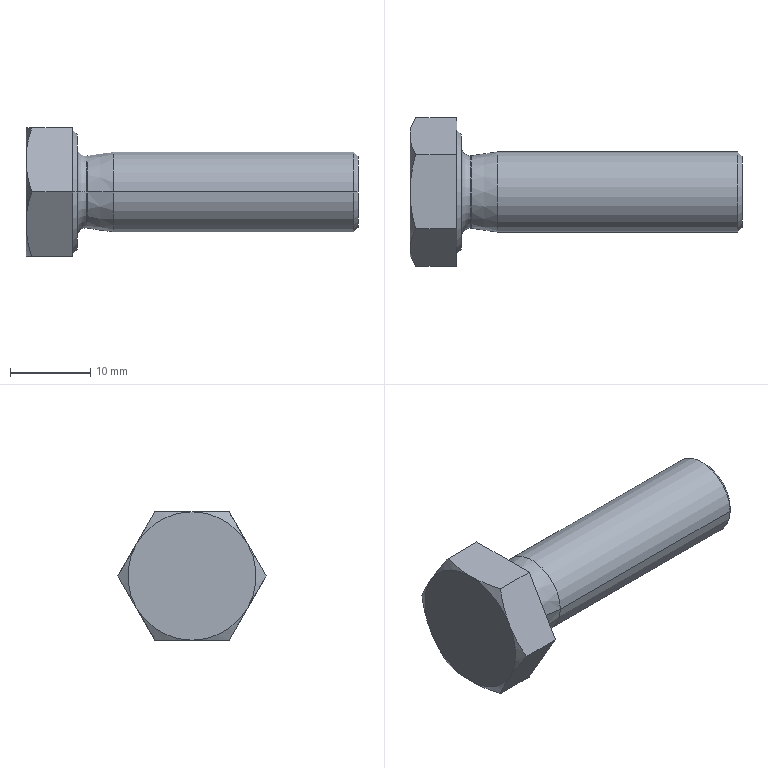Part | SolidWorks | features Chamfer 2, RevCut 2, Revolution 2, Extrusion 1, ICE 1 | 1 solid | 28 faces | box 41.4 x 18.475 x 16 mm | volume 4096 mm3 | cone 12 | plane 10 | torus 4 | cylinder 2 | commonest cylinder face diameters 10 x2
STEP:
#1=CARTESIAN_POINT('',(6.4,-5.613,0.));
#2=VERTEX_POINT('',#1);
#3=CARTESIAN_POINT('',(7.5,-4.513,0.));
#4=VERTEX_POINT('',#3);
#5=CARTESIAN_POINT('',(7.5,-5.613,0.));
#6=DIRECTION('',(0.,0.,-1.));
#7=DIRECTION('',(-1.,0.,0.));
#8=AXIS2_PLACEMENT_3D('',#5,#6,#7);
#9=CIRCLE('',#8,1.1);
#10=EDGE_CURVE('',#2,#4,#9,.T.);
#11=ORIENTED_EDGE('',*,*,#10,.T.);
#12=CARTESIAN_POINT('',(7.5,4.513,0.));
#13=VERTEX_POINT('',#12);
#14=CARTESIAN_POINT('',(7.5,0.,0.));
#15=DIRECTION('',(-1.,0.,0.));
#16=DIRECTION('',(0.,-1.,0.));
#17=AXIS2_PLACEMENT_3D('',#14,#15,#16);
#18=CIRCLE('',#17,4.513);
#19=EDGE_CURVE('',#4,#13,#18,.T.);
#20=ORIENTED_EDGE('',*,*,#19,.T.);
#21=CARTESIAN_POINT('',(6.4,5.613,0.));
#22=VERTEX_POINT('',#21);
#23=CARTESIAN_POINT('',(7.5,5.613,0.));
#24=DIRECTION('',(0.,0.,1.));
#25=DIRECTION('',(0.,-1.,0.));
#26=AXIS2_PLACEMENT_3D('',#23,#24,#25);
#27=CIRCLE('',#26,1.1);
#28=EDGE_CURVE('',#22,#13,#27,.T.);
#29=ORIENTED_EDGE('',*,*,#28,.F.);
#30=CARTESIAN_POINT('',(6.4,0.,0.));
#31=DIRECTION('',(-1.,0.,0.));
#32=DIRECTION('',(0.,-1.,0.));
#33=AXIS2_PLACEMENT_3D('',#30,#31,#32);
#34=CIRCLE('',#33,5.613);
#35=EDGE_CURVE('',#2,#22,#34,.T.);
#36=ORIENTED_EDGE('',*,*,#35,.F.);
#37=EDGE_LOOP('',(#11,#20,#29,#36));
#38=FACE_OUTER_BOUND('',#37,.T.);
#39=CARTESIAN_POINT('',(7.5,0.,0.));
#40=DIRECTION('',(-1.,0.,0.));
#41=DIRECTION('',(0.,-1.,0.));
#42=AXIS2_PLACEMENT_3D('',#39,#40,#41);
#43=TOROIDAL_SURFACE('',#42,5.613,1.1);
#44=ADVANCED_FACE('',(#38),#43,.F.);
#45=ORIENTED_EDGE('',*,*,#28,.T.);
#46=CARTESIAN_POINT('',(7.5,0.,0.));
#47=DIRECTION('',(-1.,0.,0.));
#48=DIRECTION('',(0.,-1.,0.));
#49=AXIS2_PLACEMENT_3D('',#46,#47,#48);
#50=CIRCLE('',#49,4.513);
#51=EDGE_CURVE('',#13,#4,#50,.T.);
#52=ORIENTED_EDGE('',*,*,#51,.T.);
#53=ORIENTED_EDGE('',*,*,#10,.F.);
#54=CARTESIAN_POINT('',(6.4,0.,0.));
#55=DIRECTION('',(-1.,0.,0.));
#56=DIRECTION('',(0.,-1.,0.));
#57=AXIS2_PLACEMENT_3D('',#54,#55,#56);
#58=CIRCLE('',#57,5.613);
#59=EDGE_CURVE('',#22,#2,#58,.T.);
#60=ORIENTED_EDGE('',*,*,#59,.F.);
#61=EDGE_LOOP('',(#45,#52,#53,#60));
#62=FACE_OUTER_BOUND('',#61,.T.);
#63=CARTESIAN_POINT('',(7.5,0.,0.));
#64=DIRECTION('',(-1.,0.,0.));
#65=DIRECTION('',(0.,-1.,0.));
#66=AXIS2_PLACEMENT_3D('',#63,#64,#65);
#67=TOROIDAL_SURFACE('',#66,5.613,1.1);
#68=ADVANCED_FACE('',(#62),#67,.F.);
#69=CARTESIAN_POINT('',(6.4,-7.135,0.));
#70=VERTEX_POINT('',#69);
#71=CARTESIAN_POINT('',(6.4,7.135,0.));
#72=VERTEX_POINT('',#71);
#73=CARTESIAN_POINT('',(6.4,0.,0.));
#74=DIRECTION('',(-1.,0.,0.));
#75=DIRECTION('',(0.,-1.,0.));
#76=AXIS2_PLACEMENT_3D('',#73,#74,#75);
#77=CIRCLE('',#76,7.135);
#78=EDGE_CURVE('',#70,#72,#77,.T.);
#79=ORIENTED_EDGE('',*,*,#78,.T.);
#80=CARTESIAN_POINT('',(5.8,7.735,0.));
#81=VERTEX_POINT('',#80);
#82=CARTESIAN_POINT('',(5.8,7.735,0.));
#83=DIRECTION('',(-0.7071,0.7071,0.));
#84=VECTOR('',#83,1000.);
#85=LINE('',#82,#84);
#86=EDGE_CURVE('',#72,#81,#85,.T.);
#87=ORIENTED_EDGE('',*,*,#86,.T.);
#88=CARTESIAN_POINT('',(5.8,-7.735,0.));
#89=VERTEX_POINT('',#88);
#90=CARTESIAN_POINT('',(5.8,0.,0.));
#91=DIRECTION('',(-1.,0.,0.));
#92=DIRECTION('',(0.,-1.,0.));
#93=AXIS2_PLACEMENT_3D('',#90,#91,#92);
#94=CIRCLE('',#93,7.735);
#95=EDGE_CURVE('',#89,#81,#94,.T.);
#96=ORIENTED_EDGE('',*,*,#95,.F.);
#97=CARTESIAN_POINT('',(5.8,-7.735,0.));
#98=DIRECTION('',(-0.7071,-0.7071,0.));
#99=VECTOR('',#98,1000.);
#100=LINE('',#97,#99);
#101=EDGE_CURVE('',#70,#89,#100,.T.);
#102=ORIENTED_EDGE('',*,*,#101,.F.);
#103=EDGE_LOOP('',(#79,#87,#96,#102));
#104=FACE_OUTER_BOUND('',#103,.T.);
#105=CARTESIAN_POINT('',(5.8,0.,0.));
#106=DIRECTION('',(-1.,0.,0.));
#107=DIRECTION('',(0.,-1.,0.));
#108=AXIS2_PLACEMENT_3D('',#105,#106,#107);
#109=CONICAL_SURFACE('',#108,7.735,0.7854);
#110=ADVANCED_FACE('',(#104),#109,.T.);
#111=CARTESIAN_POINT('',(41.4,4.444,0.));
#112=VERTEX_POINT('',#111);
#113=CARTESIAN_POINT('',(41.4,-4.444,0.));
#114=VERTEX_POINT('',#113);
#115=CARTESIAN_POINT('',(41.4,0.,0.));
#116=DIRECTION('',(1.,0.,0.));
#117=DIRECTION('',(0.,-1.,0.));
#118=AXIS2_PLACEMENT_3D('',#115,#116,#117);
#119=CIRCLE('',#118,4.444);
#120=EDGE_CURVE('',#112,#114,#119,.T.);
#121=ORIENTED_EDGE('',*,*,#120,.F.);
#122=CARTESIAN_POINT('',(40.844,5.,0.));
#123=VERTEX_POINT('',#122);
#124=CARTESIAN_POINT('',(40.844,5.,0.));
#125=DIRECTION('',(-0.7071,0.7071,0.));
#126=VECTOR('',#125,1000.);
#127=LINE('',#124,#126);
#128=EDGE_CURVE('',#112,#123,#127,.T.);
#129=ORIENTED_EDGE('',*,*,#128,.T.);
#130=CARTESIAN_POINT('',(40.844,-5.,0.));
#131=VERTEX_POINT('',#130);
#132=CARTESIAN_POINT('',(40.844,0.,0.));
#133=DIRECTION('',(-1.,0.,0.));
#134=DIRECTION('',(0.,-1.,0.));
#135=AXIS2_PLACEMENT_3D('',#132,#133,#134);
#136=CIRCLE('',#135,5.);
#137=EDGE_CURVE('',#131,#123,#136,.T.);
#138=ORIENTED_EDGE('',*,*,#137,.F.);
#139=CARTESIAN_POINT('',(40.844,-5.,0.));
#140=DIRECTION('',(-0.7071,-0.7071,0.));
#141=VECTOR('',#140,1000.);
#142=LINE('',#139,#141);
#143=EDGE_CURVE('',#114,#131,#142,.T.);
#144=ORIENTED_EDGE('',*,*,#143,.F.);
#145=EDGE_LOOP('',(#121,#129,#138,#144));
#146=FACE_OUTER_BOUND('',#145,.T.);
#147=CARTESIAN_POINT('',(40.844,0.,0.));
#148=DIRECTION('',(-1.,0.,0.));
#149=DIRECTION('',(0.,-1.,0.));
#150=AXIS2_PLACEMENT_3D('',#147,#148,#149);
#151=CONICAL_SURFACE('',#150,5.,0.7854);
#152=ADVANCED_FACE('',(#146),#151,.T.);
#153=ORIENTED_EDGE('',*,*,#51,.F.);
#154=CARTESIAN_POINT('',(7.66,4.525,0.));
#155=VERTEX_POINT('',#154);
#156=CARTESIAN_POINT('',(7.5,5.613,0.));
#157=DIRECTION('',(0.,0.,1.));
#158=DIRECTION('',(0.,-1.,0.));
#159=AXIS2_PLACEMENT_3D('',#156,#157,#158);
#160=CIRCLE('',#159,1.1);
#161=EDGE_CURVE('',#13,#155,#160,.T.);
#162=ORIENTED_EDGE('',*,*,#161,.T.);
#163=CARTESIAN_POINT('',(7.66,-4.525,0.));
#164=VERTEX_POINT('',#163);
#165=CARTESIAN_POINT('',(7.66,0.,0.));
#166=DIRECTION('',(-1.,0.,0.));
#167=DIRECTION('',(0.,-1.,0.));
#168=AXIS2_PLACEMENT_3D('',#165,#166,#167);
#169=CIRCLE('',#168,4.525);
#170=EDGE_CURVE('',#155,#164,#169,.T.);
#171=ORIENTED_EDGE('',*,*,#170,.T.);
#172=CARTESIAN_POINT('',(7.5,-5.613,0.));
#173=DIRECTION('',(0.,0.,-1.));
#174=DIRECTION('',(-1.,0.,0.));
#175=AXIS2_PLACEMENT_3D('',#172,#173,#174);
#176=CIRCLE('',#175,1.1);
#177=EDGE_CURVE('',#4,#164,#176,.T.);
#178=ORIENTED_EDGE('',*,*,#177,.F.);
#179=EDGE_LOOP('',(#153,#162,#171,#178));
#180=FACE_OUTER_BOUND('',#179,.T.);
#181=CARTESIAN_POINT('',(7.5,0.,0.));
#182=DIRECTION('',(-1.,0.,0.));
#183=DIRECTION('',(0.,-1.,0.));
#184=AXIS2_PLACEMENT_3D('',#181,#182,#183);
#185=TOROIDAL_SURFACE('',#184,5.613,1.1);
#186=ADVANCED_FACE('',(#180),#185,.F.);
#187=ORIENTED_EDGE('',*,*,#137,.T.);
#188=CARTESIAN_POINT('',(10.9,5.,0.));
#189=VERTEX_POINT('',#188);
#190=CARTESIAN_POINT('',(6.4,5.,0.));
#191=DIRECTION('',(-1.,0.,0.));
#192=VECTOR('',#191,1000.);
#193=LINE('',#190,#192);
#194=EDGE_CURVE('',#123,#189,#193,.T.);
#195=ORIENTED_EDGE('',*,*,#194,.T.);
#196=CARTESIAN_POINT('',(10.9,-5.,0.));
#197=VERTEX_POINT('',#196);
#198=CARTESIAN_POINT('',(10.9,0.,0.));
#199=DIRECTION('',(-1.,0.,0.));
#200=DIRECTION('',(0.,-1.,0.));
#201=AXIS2_PLACEMENT_3D('',#198,#199,#200);
#202=CIRCLE('',#201,5.);
#203=EDGE_CURVE('',#197,#189,#202,.T.);
#204=ORIENTED_EDGE('',*,*,#203,.F.);
#205=CARTESIAN_POINT('',(6.4,-5.,0.));
#206=DIRECTION('',(-1.,0.,0.));
#207=VECTOR('',#206,1000.);
#208=LINE('',#205,#207);
#209=EDGE_CURVE('',#131,#197,#208,.T.);
#210=ORIENTED_EDGE('',*,*,#209,.F.);
#211=EDGE_LOOP('',(#187,#195,#204,#210));
#212=FACE_OUTER_BOUND('',#211,.T.);
#213=CARTESIAN_POINT('',(6.4,0.,0.));
#214=DIRECTION('',(-1.,0.,0.));
#215=DIRECTION('',(0.,-1.,0.));
#216=AXIS2_PLACEMENT_3D('',#213,#214,#215);
#217=CYLINDRICAL_SURFACE('',#216,5.);
#218=ADVANCED_FACE('',(#212),#217,.T.);
#219=CARTESIAN_POINT('',(7.66,0.,0.));
#220=DIRECTION('',(-1.,0.,0.));
#221=DIRECTION('',(0.,-1.,0.));
#222=AXIS2_PLACEMENT_3D('',#219,#220,#221);
#223=CIRCLE('',#222,4.525);
#224=EDGE_CURVE('',#164,#155,#223,.T.);
#225=ORIENTED_EDGE('',*,*,#224,.F.);
#226=CARTESIAN_POINT('',(10.9,-5.,0.));
#227=DIRECTION('',(0.9894,-0.1452,0.));
#228=VECTOR('',#227,1000.);
#229=LINE('',#226,#228);
#230=EDGE_CURVE('',#164,#197,#229,.T.);
#231=ORIENTED_EDGE('',*,*,#230,.T.);
#232=ORIENTED_EDGE('',*,*,#203,.T.);
#233=CARTESIAN_POINT('',(10.9,5.,0.));
#234=DIRECTION('',(0.9894,0.1452,0.));
#235=VECTOR('',#234,1000.);
#236=LINE('',#233,#235);
#237=EDGE_CURVE('',#155,#189,#236,.T.);
#238=ORIENTED_EDGE('',*,*,#237,.F.);
#239=EDGE_LOOP('',(#225,#231,#232,#238));
#240=FACE_OUTER_BOUND('',#239,.T.);
#241=CARTESIAN_POINT('',(10.9,0.,0.));
#242=DIRECTION('',(1.,0.,0.));
#243=DIRECTION('',(0.,1.,0.));
#244=AXIS2_PLACEMENT_3D('',#241,#242,#243);
#245=CONICAL_SURFACE('',#244,5.,0.1457);
#246=ADVANCED_FACE('',(#240),#245,.T.);
#247=ORIENTED_EDGE('',*,*,#35,.T.);
#248=ORIENTED_EDGE('',*,*,#59,.T.);
#249=EDGE_LOOP('',(#247,#248));
#250=FACE_BOUND('',#249,.T.);
#251=ORIENTED_EDGE('',*,*,#78,.F.);
#252=CARTESIAN_POINT('',(6.4,0.,0.));
#253=DIRECTION('',(-1.,0.,0.));
#254=DIRECTION('',(0.,-1.,0.));
#255=AXIS2_PLACEMENT_3D('',#252,#253,#254);
#256=CIRCLE('',#255,7.135);
#257=EDGE_CURVE('',#72,#70,#256,.T.);
#258=ORIENTED_EDGE('',*,*,#257,.F.);
#259=EDGE_LOOP('',(#251,#258));
#260=FACE_OUTER_BOUND('',#259,.T.);
#261=CARTESIAN_POINT('',(6.4,4.619,-8.));
#262=DIRECTION('',(1.,0.,0.));
#263=DIRECTION('',(0.,0.,-1.));
#264=AXIS2_PLACEMENT_3D('',#261,#262,#263);
#265=PLANE('',#264);
#266=ADVANCED_FACE('',(#250,#260),#265,.T.);
#267=ORIENTED_EDGE('',*,*,#230,.F.);
#268=ORIENTED_EDGE('',*,*,#170,.F.);
#269=ORIENTED_EDGE('',*,*,#237,.T.);
#270=CARTESIAN_POINT('',(10.9,0.,0.));
#271=DIRECTION('',(-1.,0.,0.));
#272=DIRECTION('',(0.,-1.,0.));
#273=AXIS2_PLACEMENT_3D('',#270,#271,#272);
#274=CIRCLE('',#273,5.);
#275=EDGE_CURVE('',#189,#197,#274,.T.);
#276=ORIENTED_EDGE('',*,*,#275,.T.);
#277=EDGE_LOOP('',(#267,#268,#269,#276));
#278=FACE_OUTER_BOUND('',#277,.T.);
#279=CARTESIAN_POINT('',(10.9,0.,0.));
#280=DIRECTION('',(1.,0.,0.));
#281=DIRECTION('',(0.,1.,0.));
#282=AXIS2_PLACEMENT_3D('',#279,#280,#281);
#283=CONICAL_SURFACE('',#282,5.,0.1457);
#284=ADVANCED_FACE('',(#278),#283,.T.);
#285=ORIENTED_EDGE('',*,*,#194,.F.);
#286=CARTESIAN_POINT('',(40.844,0.,0.));
#287=DIRECTION('',(-1.,0.,0.));
#288=DIRECTION('',(0.,-1.,0.));
#289=AXIS2_PLACEMENT_3D('',#286,#287,#288);
#290=CIRCLE('',#289,5.);
#291=EDGE_CURVE('',#123,#131,#290,.T.);
#292=ORIENTED_EDGE('',*,*,#291,.T.);
#293=ORIENTED_EDGE('',*,*,#209,.T.);
#294=ORIENTED_EDGE('',*,*,#275,.F.);
#295=EDGE_LOOP('',(#285,#292,#293,#294));
#296=FACE_OUTER_BOUND('',#295,.T.);
#297=CARTESIAN_POINT('',(6.4,0.,0.));
#298=DIRECTION('',(-1.,0.,0.));
#299=DIRECTION('',(0.,-1.,0.));
#300=AXIS2_PLACEMENT_3D('',#297,#298,#299);
#301=CYLINDRICAL_SURFACE('',#300,5.);
#302=ADVANCED_FACE('',(#296),#301,.T.);
#303=CARTESIAN_POINT('',(41.4,0.,0.));
#304=DIRECTION('',(1.,0.,0.));
#305=DIRECTION('',(0.,-1.,0.));
#306=AXIS2_PLACEMENT_3D('',#303,#304,#305);
#307=CIRCLE('',#306,4.444);
#308=EDGE_CURVE('',#114,#112,#307,.T.);
#309=ORIENTED_EDGE('',*,*,#308,.T.);
#310=ORIENTED_EDGE('',*,*,#120,.T.);
#311=EDGE_LOOP('',(#309,#310));
#312=FACE_OUTER_BOUND('',#311,.T.);
#313=CARTESIAN_POINT('',(41.4,5.,0.));
#314=DIRECTION('',(-1.,0.,0.));
#315=DIRECTION('',(0.,-1.,0.));
#316=AXIS2_PLACEMENT_3D('',#313,#314,#315);
#317=PLANE('',#316);
#318=ADVANCED_FACE('',(#312),#317,.F.);
#319=ORIENTED_EDGE('',*,*,#19,.F.);
#320=ORIENTED_EDGE('',*,*,#177,.T.);
#321=ORIENTED_EDGE('',*,*,#224,.T.);
#322=ORIENTED_EDGE('',*,*,#161,.F.);
#323=EDGE_LOOP('',(#319,#320,#321,#322));
#324=FACE_OUTER_BOUND('',#323,.T.);
#325=CARTESIAN_POINT('',(7.5,0.,0.));
#326=DIRECTION('',(-1.,0.,0.));
#327=DIRECTION('',(0.,-1.,0.));
#328=AXIS2_PLACEMENT_3D('',#325,#326,#327);
#329=TOROIDAL_SURFACE('',#328,5.613,1.1);
#330=ADVANCED_FACE('',(#324),#329,.F.);
#331=ORIENTED_EDGE('',*,*,#128,.F.);
#332=ORIENTED_EDGE('',*,*,#308,.F.);
#333=ORIENTED_EDGE('',*,*,#143,.T.);
#334=ORIENTED_EDGE('',*,*,#291,.F.);
#335=EDGE_LOOP('',(#331,#332,#333,#334));
#336=FACE_OUTER_BOUND('',#335,.T.);
#337=CARTESIAN_POINT('',(40.844,0.,0.));
#338=DIRECTION('',(-1.,0.,0.));
#339=DIRECTION('',(0.,-1.,0.));
#340=AXIS2_PLACEMENT_3D('',#337,#338,#339);
#341=CONICAL_SURFACE('',#340,5.,0.7854);
#342=ADVANCED_FACE('',(#336),#341,.T.);
#343=ORIENTED_EDGE('',*,*,#95,.T.);
#344=CARTESIAN_POINT('',(5.8,0.,0.));
#345=DIRECTION('',(-1.,0.,0.));
#346=DIRECTION('',(0.,-1.,0.));
#347=AXIS2_PLACEMENT_3D('',#344,#345,#346);
#348=CIRCLE('',#347,7.735);
#349=EDGE_CURVE('',#81,#89,#348,.T.);
#350=ORIENTED_EDGE('',*,*,#349,.T.);
#351=EDGE_LOOP('',(#343,#350));
#352=FACE_BOUND('',#351,.T.);
#353=CARTESIAN_POINT('',(5.8,-4.619,-8.));
#354=VERTEX_POINT('',#353);
#355=CARTESIAN_POINT('',(5.8,4.619,-8.));
#356=VERTEX_POINT('',#355);
#357=CARTESIAN_POINT('',(5.8,-4.619,-8.));
#358=DIRECTION('',(0.,1.,0.));
#359=VECTOR('',#358,1000.);
#360=LINE('',#357,#359);
#361=EDGE_CURVE('',#354,#356,#360,.T.);
#362=ORIENTED_EDGE('',*,*,#361,.T.);
#363=CARTESIAN_POINT('',(5.8,9.238,0.));
#364=VERTEX_POINT('',#363);
#365=CARTESIAN_POINT('',(5.8,4.619,-8.));
#366=DIRECTION('',(0.,0.5,0.866));
#367=VECTOR('',#366,1000.);
#368=LINE('',#365,#367);
#369=EDGE_CURVE('',#356,#364,#368,.T.);
#370=ORIENTED_EDGE('',*,*,#369,.T.);
#371=CARTESIAN_POINT('',(5.8,4.619,8.));
#372=VERTEX_POINT('',#371);
#373=CARTESIAN_POINT('',(5.8,9.238,0.));
#374=DIRECTION('',(0.,-0.5,0.866));
#375=VECTOR('',#374,1000.);
#376=LINE('',#373,#375);
#377=EDGE_CURVE('',#364,#372,#376,.T.);
#378=ORIENTED_EDGE('',*,*,#377,.T.);
#379=CARTESIAN_POINT('',(5.8,-4.619,8.));
#380=VERTEX_POINT('',#379);
#381=CARTESIAN_POINT('',(5.8,4.619,8.));
#382=DIRECTION('',(0.,-1.,0.));
#383=VECTOR('',#382,1000.);
#384=LINE('',#381,#383);
#385=EDGE_CURVE('',#372,#380,#384,.T.);
#386=ORIENTED_EDGE('',*,*,#385,.T.);
#387=CARTESIAN_POINT('',(5.8,-9.238,0.));
#388=VERTEX_POINT('',#387);
#389=CARTESIAN_POINT('',(5.8,-4.619,8.));
#390=DIRECTION('',(0.,-0.5,-0.866));
#391=VECTOR('',#390,1000.);
#392=LINE('',#389,#391);
#393=EDGE_CURVE('',#380,#388,#392,.T.);
#394=ORIENTED_EDGE('',*,*,#393,.T.);
#395=CARTESIAN_POINT('',(5.8,-9.238,0.));
#396=DIRECTION('',(0.,0.5,-0.866));
#397=VECTOR('',#396,1000.);
#398=LINE('',#395,#397);
#399=EDGE_CURVE('',#388,#354,#398,.T.);
#400=ORIENTED_EDGE('',*,*,#399,.T.);
#401=EDGE_LOOP('',(#362,#370,#378,#386,#394,#400));
#402=FACE_OUTER_BOUND('',#401,.T.);
#403=CARTESIAN_POINT('',(5.8,-7.735,0.));
#404=DIRECTION('',(1.,0.,0.));
#405=DIRECTION('',(0.,1.,0.));
#406=AXIS2_PLACEMENT_3D('',#403,#404,#405);
#407=PLANE('',#406);
#408=ADVANCED_FACE('',(#352,#402),#407,.T.);
#409=ORIENTED_EDGE('',*,*,#86,.F.);
#410=ORIENTED_EDGE('',*,*,#257,.T.);
#411=ORIENTED_EDGE('',*,*,#101,.T.);
#412=ORIENTED_EDGE('',*,*,#349,.F.);
#413=EDGE_LOOP('',(#409,#410,#411,#412));
#414=FACE_OUTER_BOUND('',#413,.T.);
#415=CARTESIAN_POINT('',(5.8,0.,0.));
#416=DIRECTION('',(-1.,0.,0.));
#417=DIRECTION('',(0.,-1.,0.));
#418=AXIS2_PLACEMENT_3D('',#415,#416,#417);
#419=CONICAL_SURFACE('',#418,7.735,0.7854);
#420=ADVANCED_FACE('',(#414),#419,.T.);
#421=CARTESIAN_POINT('',(0.,0.,-8.));
#422=VERTEX_POINT('',#421);
#423=CARTESIAN_POINT('',(0.,6.928,-4.));
#424=VERTEX_POINT('',#423);
#425=CARTESIAN_POINT('',(0.,0.,0.));
#426=DIRECTION('',(1.,0.,0.));
#427=DIRECTION('',(0.,0.,-1.));
#428=AXIS2_PLACEMENT_3D('',#425,#426,#427);
#429=CIRCLE('',#428,8.);
#430=EDGE_CURVE('',#422,#424,#429,.T.);
#431=ORIENTED_EDGE('',*,*,#430,.F.);
#432=CARTESIAN_POINT('',(0.,-6.928,-4.));
#433=VERTEX_POINT('',#432);
#434=CARTESIAN_POINT('',(0.,0.,0.));
#435=DIRECTION('',(1.,0.,0.));
#436=DIRECTION('',(0.,0.,-1.));
#437=AXIS2_PLACEMENT_3D('',#434,#435,#436);
#438=CIRCLE('',#437,8.);
#439=EDGE_CURVE('',#433,#422,#438,.T.);
#440=ORIENTED_EDGE('',*,*,#439,.F.);
#441=CARTESIAN_POINT('',(0.,-6.928,4.));
#442=VERTEX_POINT('',#441);
#443=CARTESIAN_POINT('',(0.,0.,0.));
#444=DIRECTION('',(1.,0.,0.));
#445=DIRECTION('',(0.,0.,-1.));
#446=AXIS2_PLACEMENT_3D('',#443,#444,#445);
#447=CIRCLE('',#446,8.);
#448=EDGE_CURVE('',#442,#433,#447,.T.);
#449=ORIENTED_EDGE('',*,*,#448,.F.);
#450=CARTESIAN_POINT('',(0.,0.,8.));
#451=VERTEX_POINT('',#450);
#452=CARTESIAN_POINT('',(0.,0.,0.));
#453=DIRECTION('',(1.,0.,0.));
#454=DIRECTION('',(0.,0.,-1.));
#455=AXIS2_PLACEMENT_3D('',#452,#453,#454);
#456=CIRCLE('',#455,8.);
#457=EDGE_CURVE('',#451,#442,#456,.T.);
#458=ORIENTED_EDGE('',*,*,#457,.F.);
#459=CARTESIAN_POINT('',(0.,6.928,4.));
#460=VERTEX_POINT('',#459);
#461=CARTESIAN_POINT('',(0.,0.,0.));
#462=DIRECTION('',(-1.,0.,0.));
#463=DIRECTION('',(0.,0.,1.));
#464=AXIS2_PLACEMENT_3D('',#461,#462,#463);
#465=CIRCLE('',#464,8.);
#466=EDGE_CURVE('',#451,#460,#465,.T.);
#467=ORIENTED_EDGE('',*,*,#466,.T.);
#468=CARTESIAN_POINT('',(0.,0.,0.));
#469=DIRECTION('',(1.,0.,0.));
#470=DIRECTION('',(0.,0.,-1.));
#471=AXIS2_PLACEMENT_3D('',#468,#469,#470);
#472=CIRCLE('',#471,8.);
#473=EDGE_CURVE('',#424,#460,#472,.T.);
#474=ORIENTED_EDGE('',*,*,#473,.F.);
#475=EDGE_LOOP('',(#431,#440,#449,#458,#467,#474));
#476=FACE_OUTER_BOUND('',#475,.T.);
#477=CARTESIAN_POINT('',(0.,4.619,-8.));
#478=DIRECTION('',(1.,0.,0.));
#479=DIRECTION('',(0.,0.,-1.));
#480=AXIS2_PLACEMENT_3D('',#477,#478,#479);
#481=PLANE('',#480);
#482=ADVANCED_FACE('',(#476),#481,.F.);
#483=CARTESIAN_POINT('',(0.7145,4.619,-8.));
#484=VERTEX_POINT('',#483);
#485=CARTESIAN_POINT('',(0.,6.928,-4.));
#486=CARTESIAN_POINT('',(0.,6.732,-4.339));
#487=CARTESIAN_POINT('',(0.01689,6.535,-4.68));
#488=CARTESIAN_POINT('',(0.08225,6.146,-5.355));
#489=CARTESIAN_POINT('',(0.1307,5.952,-5.69));
#490=CARTESIAN_POINT('',(0.3174,5.376,-6.689));
#491=CARTESIAN_POINT('',(0.497,4.996,-7.347));
#492=CARTESIAN_POINT('',(0.7145,4.619,-8.));
#493=B_SPLINE_CURVE_WITH_KNOTS('',3,(#485,#486,#487,#488,#489,#490,#491,#492),.UNSPECIFIED.,.F.,.F.,(4,2,2,4),(0.004674,0.005838,0.007002,0.00933),.UNSPECIFIED.);
#494=EDGE_CURVE('',#424,#484,#493,.T.);
#495=ORIENTED_EDGE('',*,*,#494,.T.);
#496=CARTESIAN_POINT('',(0.7145,4.619,-8.));
#497=CARTESIAN_POINT('',(0.4989,3.872,-8.));
#498=CARTESIAN_POINT('',(0.3194,3.115,-8.));
#499=CARTESIAN_POINT('',(0.06895,1.573,-8.));
#500=CARTESIAN_POINT('',(0.,0.781,-8.));
#501=CARTESIAN_POINT('',(0.,0.,-8.));
#502=B_SPLINE_CURVE_WITH_KNOTS('',3,(#496,#497,#498,#499,#500,#501),.UNSPECIFIED.,.F.,.F.,(4,2,4),(0.003372,0.005703,0.008035),.UNSPECIFIED.);
#503=EDGE_CURVE('',#484,#422,#502,.T.);
#504=ORIENTED_EDGE('',*,*,#503,.T.);
#505=ORIENTED_EDGE('',*,*,#430,.T.);
#506=EDGE_LOOP('',(#495,#504,#505));
#507=FACE_OUTER_BOUND('',#506,.T.);
#508=CARTESIAN_POINT('',(0.,0.,0.));
#509=DIRECTION('',(1.,0.,0.));
#510=DIRECTION('',(0.,0.,1.));
#511=AXIS2_PLACEMENT_3D('',#508,#509,#510);
#512=CONICAL_SURFACE('',#511,8.,1.047);
#513=ADVANCED_FACE('',(#507),#512,.T.);
#514=CARTESIAN_POINT('',(0.7145,9.238,0.));
#515=VERTEX_POINT('',#514);
#516=CARTESIAN_POINT('',(0.,6.928,4.));
#517=CARTESIAN_POINT('',(0.,7.124,3.661));
#518=CARTESIAN_POINT('',(0.01689,7.321,3.32));
#519=CARTESIAN_POINT('',(0.08225,7.711,2.645));
#520=CARTESIAN_POINT('',(0.1307,7.904,2.31));
#521=CARTESIAN_POINT('',(0.3174,8.481,1.311));
#522=CARTESIAN_POINT('',(0.497,8.861,0.6527));
#523=CARTESIAN_POINT('',(0.7145,9.238,0.));
#524=B_SPLINE_CURVE_WITH_KNOTS('',3,(#516,#517,#518,#519,#520,#521,#522,#523),.UNSPECIFIED.,.F.,.F.,(4,2,2,4),(0.004674,0.005838,0.007002,0.00933),.UNSPECIFIED.);
#525=EDGE_CURVE('',#460,#515,#524,.T.);
#526=ORIENTED_EDGE('',*,*,#525,.T.);
#527=CARTESIAN_POINT('',(0.7145,9.238,0.));
#528=CARTESIAN_POINT('',(0.4964,8.86,-0.6543));
#529=CARTESIAN_POINT('',(0.3167,8.479,-1.313));
#530=CARTESIAN_POINT('',(0.0681,7.71,-2.646));
#531=CARTESIAN_POINT('',(0.,7.322,-3.319));
#532=CARTESIAN_POINT('',(0.,6.928,-4.));
#533=B_SPLINE_CURVE_WITH_KNOTS('',3,(#527,#528,#529,#530,#531,#532),.UNSPECIFIED.,.F.,.F.,(4,2,4),(0.000000238,0.002337,0.004674),.UNSPECIFIED.);
#534=EDGE_CURVE('',#515,#424,#533,.T.);
#535=ORIENTED_EDGE('',*,*,#534,.T.);
#536=ORIENTED_EDGE('',*,*,#473,.T.);
#537=EDGE_LOOP('',(#526,#535,#536));
#538=FACE_OUTER_BOUND('',#537,.T.);
#539=CARTESIAN_POINT('',(0.,0.,0.));
#540=DIRECTION('',(1.,0.,0.));
#541=DIRECTION('',(0.,0.,1.));
#542=AXIS2_PLACEMENT_3D('',#539,#540,#541);
#543=CONICAL_SURFACE('',#542,8.,1.047);
#544=ADVANCED_FACE('',(#538),#543,.T.);
#545=CARTESIAN_POINT('',(0.7145,4.619,8.));
#546=VERTEX_POINT('',#545);
#547=CARTESIAN_POINT('',(0.7145,4.619,8.));
#548=CARTESIAN_POINT('',(0.4964,4.997,7.346));
#549=CARTESIAN_POINT('',(0.3167,5.377,6.687));
#550=CARTESIAN_POINT('',(0.0681,6.146,5.354));
#551=CARTESIAN_POINT('',(0.,6.535,4.681));
#552=CARTESIAN_POINT('',(0.,6.928,4.));
#553=B_SPLINE_CURVE_WITH_KNOTS('',3,(#547,#548,#549,#550,#551,#552),.UNSPECIFIED.,.F.,.F.,(4,2,4),(0.000000238,0.002337,0.004674),.UNSPECIFIED.);
#554=EDGE_CURVE('',#546,#460,#553,.T.);
#555=ORIENTED_EDGE('',*,*,#554,.T.);
#556=ORIENTED_EDGE('',*,*,#466,.F.);
#557=CARTESIAN_POINT('',(0.,0.,8.));
#558=CARTESIAN_POINT('',(0.,0.781,8.));
#559=CARTESIAN_POINT('',(0.06895,1.573,8.));
#560=CARTESIAN_POINT('',(0.3194,3.115,8.));
#561=CARTESIAN_POINT('',(0.4989,3.872,8.));
#562=CARTESIAN_POINT('',(0.7145,4.619,8.));
#563=B_SPLINE_CURVE_WITH_KNOTS('',3,(#557,#558,#559,#560,#561,#562),.UNSPECIFIED.,.F.,.F.,(4,2,4),(0.01293,0.01526,0.0176),.UNSPECIFIED.);
#564=EDGE_CURVE('',#451,#546,#563,.T.);
#565=ORIENTED_EDGE('',*,*,#564,.T.);
#566=EDGE_LOOP('',(#555,#556,#565));
#567=FACE_OUTER_BOUND('',#566,.T.);
#568=CARTESIAN_POINT('',(0.,0.,0.));
#569=DIRECTION('',(1.,0.,0.));
#570=DIRECTION('',(0.,0.,1.));
#571=AXIS2_PLACEMENT_3D('',#568,#569,#570);
#572=CONICAL_SURFACE('',#571,8.,1.047);
#573=ADVANCED_FACE('',(#567),#572,.T.);
#574=CARTESIAN_POINT('',(0.7145,-4.619,8.));
#575=VERTEX_POINT('',#574);
#576=CARTESIAN_POINT('',(0.7145,-4.619,8.));
#577=CARTESIAN_POINT('',(0.4977,-3.868,8.));
#578=CARTESIAN_POINT('',(0.3158,-3.098,8.));
#579=CARTESIAN_POINT('',(0.06709,-1.556,8.));
#580=CARTESIAN_POINT('',(0.,-0.7805,8.));
#581=CARTESIAN_POINT('',(0.,0.,8.));
#582=B_SPLINE_CURVE_WITH_KNOTS('',3,(#576,#577,#578,#579,#580,#581),.UNSPECIFIED.,.F.,.F.,(4,2,4),(0.008254,0.01059,0.01293),.UNSPECIFIED.);
#583=EDGE_CURVE('',#575,#451,#582,.T.);
#584=ORIENTED_EDGE('',*,*,#583,.T.);
#585=ORIENTED_EDGE('',*,*,#457,.T.);
#586=CARTESIAN_POINT('',(0.,-6.928,4.));
#587=CARTESIAN_POINT('',(0.,-6.732,4.339));
#588=CARTESIAN_POINT('',(0.01689,-6.535,4.68));
#589=CARTESIAN_POINT('',(0.08225,-6.146,5.355));
#590=CARTESIAN_POINT('',(0.1307,-5.952,5.69));
#591=CARTESIAN_POINT('',(0.3174,-5.376,6.689));
#592=CARTESIAN_POINT('',(0.497,-4.996,7.347));
#593=CARTESIAN_POINT('',(0.7145,-4.619,8.));
#594=B_SPLINE_CURVE_WITH_KNOTS('',3,(#586,#587,#588,#589,#590,#591,#592,#593),.UNSPECIFIED.,.F.,.F.,(4,2,2,4),(0.004674,0.005838,0.007002,0.00933),.UNSPECIFIED.);
#595=EDGE_CURVE('',#442,#575,#594,.T.);
#596=ORIENTED_EDGE('',*,*,#595,.T.);
#597=EDGE_LOOP('',(#584,#585,#596));
#598=FACE_OUTER_BOUND('',#597,.T.);
#599=CARTESIAN_POINT('',(0.,0.,0.));
#600=DIRECTION('',(1.,0.,0.));
#601=DIRECTION('',(0.,0.,1.));
#602=AXIS2_PLACEMENT_3D('',#599,#600,#601);
#603=CONICAL_SURFACE('',#602,8.,1.047);
#604=ADVANCED_FACE('',(#598),#603,.T.);
#605=CARTESIAN_POINT('',(0.7145,-4.619,-8.));
#606=VERTEX_POINT('',#605);
#607=CARTESIAN_POINT('',(0.,0.,-8.));
#608=CARTESIAN_POINT('',(0.,-0.7805,-8.));
#609=CARTESIAN_POINT('',(0.06709,-1.556,-8.));
#610=CARTESIAN_POINT('',(0.3158,-3.098,-8.));
#611=CARTESIAN_POINT('',(0.4977,-3.868,-8.));
#612=CARTESIAN_POINT('',(0.7145,-4.619,-8.));
#613=B_SPLINE_CURVE_WITH_KNOTS('',3,(#607,#608,#609,#610,#611,#612),.UNSPECIFIED.,.F.,.F.,(4,2,4),(0.008035,0.01037,0.0127),.UNSPECIFIED.);
#614=EDGE_CURVE('',#422,#606,#613,.T.);
#615=ORIENTED_EDGE('',*,*,#614,.T.);
#616=CARTESIAN_POINT('',(0.7145,-4.619,-8.));
#617=CARTESIAN_POINT('',(0.4964,-4.997,-7.346));
#618=CARTESIAN_POINT('',(0.3167,-5.377,-6.687));
#619=CARTESIAN_POINT('',(0.0681,-6.146,-5.354));
#620=CARTESIAN_POINT('',(0.,-6.535,-4.681));
#621=CARTESIAN_POINT('',(0.,-6.928,-4.));
#622=B_SPLINE_CURVE_WITH_KNOTS('',3,(#616,#617,#618,#619,#620,#621),.UNSPECIFIED.,.F.,.F.,(4,2,4),(0.000000238,0.002337,0.004674),.UNSPECIFIED.);
#623=EDGE_CURVE('',#606,#433,#622,.T.);
#624=ORIENTED_EDGE('',*,*,#623,.T.);
#625=ORIENTED_EDGE('',*,*,#439,.T.);
#626=EDGE_LOOP('',(#615,#624,#625));
#627=FACE_OUTER_BOUND('',#626,.T.);
#628=CARTESIAN_POINT('',(0.,0.,0.));
#629=DIRECTION('',(1.,0.,0.));
#630=DIRECTION('',(0.,0.,1.));
#631=AXIS2_PLACEMENT_3D('',#628,#629,#630);
#632=CONICAL_SURFACE('',#631,8.,1.047);
#633=ADVANCED_FACE('',(#627),#632,.T.);
#634=CARTESIAN_POINT('',(0.7145,-9.238,0.));
#635=VERTEX_POINT('',#634);
#636=CARTESIAN_POINT('',(0.7145,-9.238,0.));
#637=CARTESIAN_POINT('',(0.4964,-8.86,0.6543));
#638=CARTESIAN_POINT('',(0.3167,-8.479,1.313));
#639=CARTESIAN_POINT('',(0.0681,-7.71,2.646));
#640=CARTESIAN_POINT('',(0.,-7.322,3.319));
#641=CARTESIAN_POINT('',(0.,-6.928,4.));
#642=B_SPLINE_CURVE_WITH_KNOTS('',3,(#636,#637,#638,#639,#640,#641),.UNSPECIFIED.,.F.,.F.,(4,2,4),(0.000000238,0.002337,0.004674),.UNSPECIFIED.);
#643=EDGE_CURVE('',#635,#442,#642,.T.);
#644=ORIENTED_EDGE('',*,*,#643,.T.);
#645=ORIENTED_EDGE('',*,*,#448,.T.);
#646=CARTESIAN_POINT('',(0.,-6.928,-4.));
#647=CARTESIAN_POINT('',(0.,-7.124,-3.661));
#648=CARTESIAN_POINT('',(0.01689,-7.321,-3.32));
#649=CARTESIAN_POINT('',(0.08225,-7.711,-2.645));
#650=CARTESIAN_POINT('',(0.1307,-7.904,-2.31));
#651=CARTESIAN_POINT('',(0.3174,-8.481,-1.311));
#652=CARTESIAN_POINT('',(0.497,-8.861,-0.6527));
#653=CARTESIAN_POINT('',(0.7145,-9.238,0.));
#654=B_SPLINE_CURVE_WITH_KNOTS('',3,(#646,#647,#648,#649,#650,#651,#652,#653),.UNSPECIFIED.,.F.,.F.,(4,2,2,4),(0.004674,0.005838,0.007002,0.00933),.UNSPECIFIED.);
#655=EDGE_CURVE('',#433,#635,#654,.T.);
#656=ORIENTED_EDGE('',*,*,#655,.T.);
#657=EDGE_LOOP('',(#644,#645,#656));
#658=FACE_OUTER_BOUND('',#657,.T.);
#659=CARTESIAN_POINT('',(0.,0.,0.));
#660=DIRECTION('',(1.,0.,0.));
#661=DIRECTION('',(0.,0.,1.));
#662=AXIS2_PLACEMENT_3D('',#659,#660,#661);
#663=CONICAL_SURFACE('',#662,8.,1.047);
#664=ADVANCED_FACE('',(#658),#663,.T.);
#665=ORIENTED_EDGE('',*,*,#399,.F.);
#666=CARTESIAN_POINT('',(6.4,-9.238,0.));
#667=DIRECTION('',(-1.,0.,0.));
#668=VECTOR('',#667,1000.);
#669=LINE('',#666,#668);
#670=EDGE_CURVE('',#388,#635,#669,.T.);
#671=ORIENTED_EDGE('',*,*,#670,.T.);
#672=ORIENTED_EDGE('',*,*,#655,.F.);
#673=ORIENTED_EDGE('',*,*,#623,.F.);
#674=CARTESIAN_POINT('',(6.4,-4.619,-8.));
#675=DIRECTION('',(-1.,0.,0.));
#676=VECTOR('',#675,1000.);
#677=LINE('',#674,#676);
#678=EDGE_CURVE('',#354,#606,#677,.T.);
#679=ORIENTED_EDGE('',*,*,#678,.F.);
#680=EDGE_LOOP('',(#665,#671,#672,#673,#679));
#681=FACE_OUTER_BOUND('',#680,.T.);
#682=CARTESIAN_POINT('',(6.4,-9.238,0.));
#683=DIRECTION('',(0.,0.866,0.5));
#684=DIRECTION('',(0.,-0.5,0.866));
#685=AXIS2_PLACEMENT_3D('',#682,#683,#684);
#686=PLANE('',#685);
#687=ADVANCED_FACE('',(#681),#686,.F.);
#688=ORIENTED_EDGE('',*,*,#393,.F.);
#689=CARTESIAN_POINT('',(6.4,-4.619,8.));
#690=DIRECTION('',(-1.,0.,0.));
#691=VECTOR('',#690,1000.);
#692=LINE('',#689,#691);
#693=EDGE_CURVE('',#380,#575,#692,.T.);
#694=ORIENTED_EDGE('',*,*,#693,.T.);
#695=ORIENTED_EDGE('',*,*,#595,.F.);
#696=ORIENTED_EDGE('',*,*,#643,.F.);
#697=ORIENTED_EDGE('',*,*,#670,.F.);
#698=EDGE_LOOP('',(#688,#694,#695,#696,#697));
#699=FACE_OUTER_BOUND('',#698,.T.);
#700=CARTESIAN_POINT('',(6.4,-4.619,8.));
#701=DIRECTION('',(0.,0.866,-0.5));
#702=DIRECTION('',(0.,0.5,0.866));
#703=AXIS2_PLACEMENT_3D('',#700,#701,#702);
#704=PLANE('',#703);
#705=ADVANCED_FACE('',(#699),#704,.F.);
#706=ORIENTED_EDGE('',*,*,#385,.F.);
#707=CARTESIAN_POINT('',(6.4,4.619,8.));
#708=DIRECTION('',(-1.,0.,0.));
#709=VECTOR('',#708,1000.);
#710=LINE('',#707,#709);
#711=EDGE_CURVE('',#372,#546,#710,.T.);
#712=ORIENTED_EDGE('',*,*,#711,.T.);
#713=ORIENTED_EDGE('',*,*,#564,.F.);
#714=ORIENTED_EDGE('',*,*,#583,.F.);
#715=ORIENTED_EDGE('',*,*,#693,.F.);
#716=EDGE_LOOP('',(#706,#712,#713,#714,#715));
#717=FACE_OUTER_BOUND('',#716,.T.);
#718=CARTESIAN_POINT('',(6.4,4.619,8.));
#719=DIRECTION('',(0.,0.,-1.));
#720=DIRECTION('',(-1.,0.,0.));
#721=AXIS2_PLACEMENT_3D('',#718,#719,#720);
#722=PLANE('',#721);
#723=ADVANCED_FACE('',(#717),#722,.F.);
#724=ORIENTED_EDGE('',*,*,#377,.F.);
#725=CARTESIAN_POINT('',(6.4,9.238,0.));
#726=DIRECTION('',(-1.,0.,0.));
#727=VECTOR('',#726,1000.);
#728=LINE('',#725,#727);
#729=EDGE_CURVE('',#364,#515,#728,.T.);
#730=ORIENTED_EDGE('',*,*,#729,.T.);
#731=ORIENTED_EDGE('',*,*,#525,.F.);
#732=ORIENTED_EDGE('',*,*,#554,.F.);
#733=ORIENTED_EDGE('',*,*,#711,.F.);
#734=EDGE_LOOP('',(#724,#730,#731,#732,#733));
#735=FACE_OUTER_BOUND('',#734,.T.);
#736=CARTESIAN_POINT('',(6.4,9.238,0.));
#737=DIRECTION('',(0.,-0.866,-0.5));
#738=DIRECTION('',(0.,0.5,-0.866));
#739=AXIS2_PLACEMENT_3D('',#736,#737,#738);
#740=PLANE('',#739);
#741=ADVANCED_FACE('',(#735),#740,.F.);
#742=ORIENTED_EDGE('',*,*,#369,.F.);
#743=CARTESIAN_POINT('',(6.4,4.619,-8.));
#744=DIRECTION('',(-1.,0.,0.));
#745=VECTOR('',#744,1000.);
#746=LINE('',#743,#745);
#747=EDGE_CURVE('',#356,#484,#746,.T.);
#748=ORIENTED_EDGE('',*,*,#747,.T.);
#749=ORIENTED_EDGE('',*,*,#494,.F.);
#750=ORIENTED_EDGE('',*,*,#534,.F.);
#751=ORIENTED_EDGE('',*,*,#729,.F.);
#752=EDGE_LOOP('',(#742,#748,#749,#750,#751));
#753=FACE_OUTER_BOUND('',#752,.T.);
#754=CARTESIAN_POINT('',(6.4,4.619,-8.));
#755=DIRECTION('',(0.,-0.866,0.5));
#756=DIRECTION('',(0.,-0.5,-0.866));
#757=AXIS2_PLACEMENT_3D('',#754,#755,#756);
#758=PLANE('',#757);
#759=ADVANCED_FACE('',(#753),#758,.F.);
#760=ORIENTED_EDGE('',*,*,#361,.F.);
#761=ORIENTED_EDGE('',*,*,#678,.T.);
#762=ORIENTED_EDGE('',*,*,#614,.F.);
#763=ORIENTED_EDGE('',*,*,#503,.F.);
#764=ORIENTED_EDGE('',*,*,#747,.F.);
#765=EDGE_LOOP('',(#760,#761,#762,#763,#764));
#766=FACE_OUTER_BOUND('',#765,.T.);
#767=CARTESIAN_POINT('',(6.4,-4.619,-8.));
#768=DIRECTION('',(0.,0.,1.));
#769=DIRECTION('',(0.,-1.,0.));
#770=AXIS2_PLACEMENT_3D('',#767,#768,#769);
#771=PLANE('',#770);
#772=ADVANCED_FACE('',(#766),#771,.F.);
#773=CLOSED_SHELL('',(#44,#68,#110,#152,#186,#218,#246,#266,#284,#302,#318,#330,#342,#408,#420,#482,#513,#544,#573,#604,#633,#664,#687,#705,#723,#741,#759,#772));
#774=MANIFOLD_SOLID_BREP('',#773);
#775=CARTESIAN_POINT('',(0.,0.,0.));
#776=DIRECTION('',(0.,0.,1.));
#777=DIRECTION('',(1.,0.,0.));
#778=AXIS2_PLACEMENT_3D('',#775,#776,#777);
#779=(LENGTH_UNIT()NAMED_UNIT(*)SI_UNIT(.MILLI.,.METRE.));
#780=UNCERTAINTY_MEASURE_WITH_UNIT(LENGTH_MEASURE(0.00001),#779,'','');
#781=(NAMED_UNIT(*)PLANE_ANGLE_UNIT()SI_UNIT($,.RADIAN.));
#782=(NAMED_UNIT(*)SI_UNIT($,.STERADIAN.)SOLID_ANGLE_UNIT());
#783=(GEOMETRIC_REPRESENTATION_CONTEXT(3)GLOBAL_UNCERTAINTY_ASSIGNED_CONTEXT((#780))GLOBAL_UNIT_ASSIGNED_CONTEXT((#779,#781,#782))REPRESENTATION_CONTEXT('',''));
#784=ADVANCED_BREP_SHAPE_REPRESENTATION('',(#774,#778),#783);